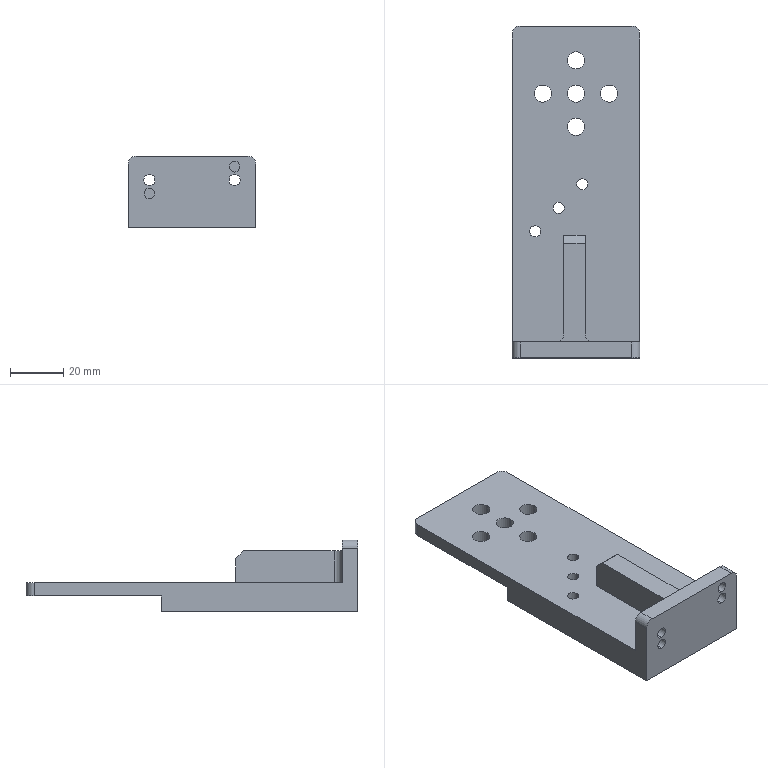Part | 1 solid | 47 faces | box 48 x 124.7 x 27 mm | volume 58099 mm3 | cylinder 30 | plane 17 | commonest cylinder face diameters 4.2 x10 6.5 x10 6 x6 4 x4
STEP:
#1=CARTESIAN_POINT('',(-17.439,-14.789,-27.));
#2=VERTEX_POINT('',#1);
#3=CARTESIAN_POINT('',(-13.239,-14.789,-27.));
#4=VERTEX_POINT('',#3);
#5=CARTESIAN_POINT('',(-15.339,-14.789,-27.));
#6=DIRECTION('',(0.,0.,1.));
#7=DIRECTION('',(1.,0.,0.));
#8=AXIS2_PLACEMENT_3D('',#5,#6,#7);
#9=CIRCLE('',#8,2.1);
#10=EDGE_CURVE('',#2,#4,#9,.T.);
#11=ORIENTED_EDGE('',*,*,#10,.F.);
#12=CARTESIAN_POINT('',(-17.439,-14.789,-16.));
#13=VERTEX_POINT('',#12);
#14=CARTESIAN_POINT('',(-17.439,-14.789,-27.));
#15=DIRECTION('',(0.,0.,1.));
#16=VECTOR('',#15,1000.);
#17=LINE('',#14,#16);
#18=EDGE_CURVE('',#13,#2,#17,.F.);
#19=ORIENTED_EDGE('',*,*,#18,.F.);
#20=CARTESIAN_POINT('',(-13.239,-14.789,-16.));
#21=VERTEX_POINT('',#20);
#22=CARTESIAN_POINT('',(-15.339,-14.789,-16.));
#23=DIRECTION('',(0.,0.,1.));
#24=DIRECTION('',(1.,0.,0.));
#25=AXIS2_PLACEMENT_3D('',#22,#23,#24);
#26=CIRCLE('',#25,2.1);
#27=EDGE_CURVE('',#13,#21,#26,.T.);
#28=ORIENTED_EDGE('',*,*,#27,.T.);
#29=CARTESIAN_POINT('',(-13.239,-14.789,-27.));
#30=DIRECTION('',(0.,0.,1.));
#31=VECTOR('',#30,1000.);
#32=LINE('',#29,#31);
#33=EDGE_CURVE('',#21,#4,#32,.F.);
#34=ORIENTED_EDGE('',*,*,#33,.T.);
#35=EDGE_LOOP('',(#11,#19,#28,#34));
#36=FACE_BOUND('',#35,.T.);
#37=CARTESIAN_POINT('',(-15.339,-14.789,-27.));
#38=DIRECTION('',(0.,0.,1.));
#39=DIRECTION('',(-1.,0.,0.));
#40=AXIS2_PLACEMENT_3D('',#37,#38,#39);
#41=CYLINDRICAL_SURFACE('',#40,2.1);
#42=ADVANCED_FACE('',(#36),#41,.F.);
#43=CARTESIAN_POINT('',(0.2388,2.889,-27.));
#44=VERTEX_POINT('',#43);
#45=CARTESIAN_POINT('',(4.439,2.889,-27.));
#46=VERTEX_POINT('',#45);
#47=CARTESIAN_POINT('',(2.339,2.889,-27.));
#48=DIRECTION('',(0.,0.,1.));
#49=DIRECTION('',(1.,0.,0.));
#50=AXIS2_PLACEMENT_3D('',#47,#48,#49);
#51=CIRCLE('',#50,2.1);
#52=EDGE_CURVE('',#44,#46,#51,.T.);
#53=ORIENTED_EDGE('',*,*,#52,.F.);
#54=CARTESIAN_POINT('',(0.2388,2.889,-16.));
#55=VERTEX_POINT('',#54);
#56=CARTESIAN_POINT('',(0.2388,2.889,-27.));
#57=DIRECTION('',(0.,0.,1.));
#58=VECTOR('',#57,1000.);
#59=LINE('',#56,#58);
#60=EDGE_CURVE('',#55,#44,#59,.F.);
#61=ORIENTED_EDGE('',*,*,#60,.F.);
#62=CARTESIAN_POINT('',(4.439,2.889,-16.));
#63=VERTEX_POINT('',#62);
#64=CARTESIAN_POINT('',(2.339,2.889,-16.));
#65=DIRECTION('',(0.,0.,1.));
#66=DIRECTION('',(1.,0.,0.));
#67=AXIS2_PLACEMENT_3D('',#64,#65,#66);
#68=CIRCLE('',#67,2.1);
#69=EDGE_CURVE('',#55,#63,#68,.T.);
#70=ORIENTED_EDGE('',*,*,#69,.T.);
#71=CARTESIAN_POINT('',(4.439,2.889,-27.));
#72=DIRECTION('',(0.,0.,1.));
#73=VECTOR('',#72,1000.);
#74=LINE('',#71,#73);
#75=EDGE_CURVE('',#63,#46,#74,.F.);
#76=ORIENTED_EDGE('',*,*,#75,.T.);
#77=EDGE_LOOP('',(#53,#61,#70,#76));
#78=FACE_BOUND('',#77,.T.);
#79=CARTESIAN_POINT('',(2.339,2.889,-27.));
#80=DIRECTION('',(0.,0.,1.));
#81=DIRECTION('',(-1.,0.,0.));
#82=AXIS2_PLACEMENT_3D('',#79,#80,#81);
#83=CYLINDRICAL_SURFACE('',#82,2.1);
#84=ADVANCED_FACE('',(#78),#83,.F.);
#85=CARTESIAN_POINT('',(-8.6,-5.95,-27.));
#86=VERTEX_POINT('',#85);
#87=CARTESIAN_POINT('',(-4.4,-5.95,-27.));
#88=VERTEX_POINT('',#87);
#89=CARTESIAN_POINT('',(-6.5,-5.95,-27.));
#90=DIRECTION('',(0.,0.,1.));
#91=DIRECTION('',(1.,0.,0.));
#92=AXIS2_PLACEMENT_3D('',#89,#90,#91);
#93=CIRCLE('',#92,2.1);
#94=EDGE_CURVE('',#86,#88,#93,.T.);
#95=ORIENTED_EDGE('',*,*,#94,.F.);
#96=CARTESIAN_POINT('',(-8.6,-5.95,-16.));
#97=VERTEX_POINT('',#96);
#98=CARTESIAN_POINT('',(-8.6,-5.95,-27.));
#99=DIRECTION('',(0.,0.,1.));
#100=VECTOR('',#99,1000.);
#101=LINE('',#98,#100);
#102=EDGE_CURVE('',#97,#86,#101,.F.);
#103=ORIENTED_EDGE('',*,*,#102,.F.);
#104=CARTESIAN_POINT('',(-4.4,-5.95,-16.));
#105=VERTEX_POINT('',#104);
#106=CARTESIAN_POINT('',(-6.5,-5.95,-16.));
#107=DIRECTION('',(0.,0.,1.));
#108=DIRECTION('',(1.,0.,0.));
#109=AXIS2_PLACEMENT_3D('',#106,#107,#108);
#110=CIRCLE('',#109,2.1);
#111=EDGE_CURVE('',#97,#105,#110,.T.);
#112=ORIENTED_EDGE('',*,*,#111,.T.);
#113=CARTESIAN_POINT('',(-4.4,-5.95,-27.));
#114=DIRECTION('',(0.,0.,1.));
#115=VECTOR('',#114,1000.);
#116=LINE('',#113,#115);
#117=EDGE_CURVE('',#105,#88,#116,.F.);
#118=ORIENTED_EDGE('',*,*,#117,.T.);
#119=EDGE_LOOP('',(#95,#103,#112,#118));
#120=FACE_BOUND('',#119,.T.);
#121=CARTESIAN_POINT('',(-6.5,-5.95,-27.));
#122=DIRECTION('',(0.,0.,1.));
#123=DIRECTION('',(-1.,0.,0.));
#124=AXIS2_PLACEMENT_3D('',#121,#122,#123);
#125=CYLINDRICAL_SURFACE('',#124,2.1);
#126=ADVANCED_FACE('',(#120),#125,.F.);
#127=CARTESIAN_POINT('',(16.,-59.35,-6.));
#128=VERTEX_POINT('',#127);
#129=CARTESIAN_POINT('',(16.,-59.35,-2.));
#130=VERTEX_POINT('',#129);
#131=CARTESIAN_POINT('',(16.,-59.35,-4.));
#132=DIRECTION('',(0.,-1.,0.));
#133=DIRECTION('',(0.,0.,1.));
#134=AXIS2_PLACEMENT_3D('',#131,#132,#133);
#135=CIRCLE('',#134,2.);
#136=EDGE_CURVE('',#128,#130,#135,.T.);
#137=ORIENTED_EDGE('',*,*,#136,.F.);
#138=CARTESIAN_POINT('',(16.,-62.35,-6.));
#139=VERTEX_POINT('',#138);
#140=CARTESIAN_POINT('',(16.,-59.35,-6.));
#141=DIRECTION('',(0.,-1.,0.));
#142=VECTOR('',#141,1000.);
#143=LINE('',#140,#142);
#144=EDGE_CURVE('',#139,#128,#143,.F.);
#145=ORIENTED_EDGE('',*,*,#144,.F.);
#146=CARTESIAN_POINT('',(16.,-62.35,-2.));
#147=VERTEX_POINT('',#146);
#148=CARTESIAN_POINT('',(16.,-62.35,-4.));
#149=DIRECTION('',(0.,-1.,0.));
#150=DIRECTION('',(0.,0.,1.));
#151=AXIS2_PLACEMENT_3D('',#148,#149,#150);
#152=CIRCLE('',#151,2.);
#153=EDGE_CURVE('',#139,#147,#152,.T.);
#154=ORIENTED_EDGE('',*,*,#153,.T.);
#155=CARTESIAN_POINT('',(16.,-59.35,-2.));
#156=DIRECTION('',(0.,-1.,0.));
#157=VECTOR('',#156,1000.);
#158=LINE('',#155,#157);
#159=EDGE_CURVE('',#147,#130,#158,.F.);
#160=ORIENTED_EDGE('',*,*,#159,.T.);
#161=EDGE_LOOP('',(#137,#145,#154,#160));
#162=FACE_BOUND('',#161,.T.);
#163=CARTESIAN_POINT('',(16.,-59.35,-4.));
#164=DIRECTION('',(0.,-1.,0.));
#165=DIRECTION('',(0.,0.,-1.));
#166=AXIS2_PLACEMENT_3D('',#163,#164,#165);
#167=CYLINDRICAL_SURFACE('',#166,2.);
#168=ADVANCED_FACE('',(#162),#167,.F.);
#169=CARTESIAN_POINT('',(-16.,-59.35,-16.));
#170=VERTEX_POINT('',#169);
#171=CARTESIAN_POINT('',(-16.,-59.35,-12.));
#172=VERTEX_POINT('',#171);
#173=CARTESIAN_POINT('',(-16.,-59.35,-14.));
#174=DIRECTION('',(0.,-1.,0.));
#175=DIRECTION('',(0.,0.,1.));
#176=AXIS2_PLACEMENT_3D('',#173,#174,#175);
#177=CIRCLE('',#176,2.);
#178=EDGE_CURVE('',#170,#172,#177,.T.);
#179=ORIENTED_EDGE('',*,*,#178,.F.);
#180=CARTESIAN_POINT('',(-16.,-62.35,-16.));
#181=VERTEX_POINT('',#180);
#182=CARTESIAN_POINT('',(-16.,-59.35,-16.));
#183=DIRECTION('',(0.,-1.,0.));
#184=VECTOR('',#183,1000.);
#185=LINE('',#182,#184);
#186=EDGE_CURVE('',#181,#170,#185,.F.);
#187=ORIENTED_EDGE('',*,*,#186,.F.);
#188=CARTESIAN_POINT('',(-16.,-62.35,-12.));
#189=VERTEX_POINT('',#188);
#190=CARTESIAN_POINT('',(-16.,-62.35,-14.));
#191=DIRECTION('',(0.,-1.,0.));
#192=DIRECTION('',(0.,0.,1.));
#193=AXIS2_PLACEMENT_3D('',#190,#191,#192);
#194=CIRCLE('',#193,2.);
#195=EDGE_CURVE('',#181,#189,#194,.T.);
#196=ORIENTED_EDGE('',*,*,#195,.T.);
#197=CARTESIAN_POINT('',(-16.,-59.35,-12.));
#198=DIRECTION('',(0.,-1.,0.));
#199=VECTOR('',#198,1000.);
#200=LINE('',#197,#199);
#201=EDGE_CURVE('',#189,#172,#200,.F.);
#202=ORIENTED_EDGE('',*,*,#201,.T.);
#203=EDGE_LOOP('',(#179,#187,#196,#202));
#204=FACE_BOUND('',#203,.T.);
#205=CARTESIAN_POINT('',(-16.,-59.35,-14.));
#206=DIRECTION('',(0.,-1.,0.));
#207=DIRECTION('',(0.,0.,-1.));
#208=AXIS2_PLACEMENT_3D('',#205,#206,#207);
#209=CYLINDRICAL_SURFACE('',#208,2.);
#210=ADVANCED_FACE('',(#204),#209,.F.);
#211=CARTESIAN_POINT('',(-3.25,49.45,-21.));
#212=VERTEX_POINT('',#211);
#213=CARTESIAN_POINT('',(3.25,49.45,-21.));
#214=VERTEX_POINT('',#213);
#215=CARTESIAN_POINT('',(0.,49.45,-21.));
#216=DIRECTION('',(0.,0.,1.));
#217=DIRECTION('',(1.,0.,0.));
#218=AXIS2_PLACEMENT_3D('',#215,#216,#217);
#219=CIRCLE('',#218,3.25);
#220=EDGE_CURVE('',#212,#214,#219,.T.);
#221=ORIENTED_EDGE('',*,*,#220,.F.);
#222=CARTESIAN_POINT('',(-3.25,49.45,-16.));
#223=VERTEX_POINT('',#222);
#224=CARTESIAN_POINT('',(-3.25,49.45,-27.));
#225=DIRECTION('',(0.,0.,1.));
#226=VECTOR('',#225,1000.);
#227=LINE('',#224,#226);
#228=EDGE_CURVE('',#223,#212,#227,.F.);
#229=ORIENTED_EDGE('',*,*,#228,.F.);
#230=CARTESIAN_POINT('',(3.25,49.45,-16.));
#231=VERTEX_POINT('',#230);
#232=CARTESIAN_POINT('',(0.,49.45,-16.));
#233=DIRECTION('',(0.,0.,1.));
#234=DIRECTION('',(1.,0.,0.));
#235=AXIS2_PLACEMENT_3D('',#232,#233,#234);
#236=CIRCLE('',#235,3.25);
#237=EDGE_CURVE('',#223,#231,#236,.T.);
#238=ORIENTED_EDGE('',*,*,#237,.T.);
#239=CARTESIAN_POINT('',(3.25,49.45,-27.));
#240=DIRECTION('',(0.,0.,1.));
#241=VECTOR('',#240,1000.);
#242=LINE('',#239,#241);
#243=EDGE_CURVE('',#231,#214,#242,.F.);
#244=ORIENTED_EDGE('',*,*,#243,.T.);
#245=EDGE_LOOP('',(#221,#229,#238,#244));
#246=FACE_BOUND('',#245,.T.);
#247=CARTESIAN_POINT('',(0.,49.45,-27.));
#248=DIRECTION('',(0.,0.,1.));
#249=DIRECTION('',(-1.,0.,0.));
#250=AXIS2_PLACEMENT_3D('',#247,#248,#249);
#251=CYLINDRICAL_SURFACE('',#250,3.25);
#252=ADVANCED_FACE('',(#246),#251,.F.);
#253=CARTESIAN_POINT('',(-15.75,36.95,-21.));
#254=VERTEX_POINT('',#253);
#255=CARTESIAN_POINT('',(-9.25,36.95,-21.));
#256=VERTEX_POINT('',#255);
#257=CARTESIAN_POINT('',(-12.5,36.95,-21.));
#258=DIRECTION('',(0.,0.,1.));
#259=DIRECTION('',(1.,0.,0.));
#260=AXIS2_PLACEMENT_3D('',#257,#258,#259);
#261=CIRCLE('',#260,3.25);
#262=EDGE_CURVE('',#254,#256,#261,.T.);
#263=ORIENTED_EDGE('',*,*,#262,.F.);
#264=CARTESIAN_POINT('',(-15.75,36.95,-16.));
#265=VERTEX_POINT('',#264);
#266=CARTESIAN_POINT('',(-15.75,36.95,-27.));
#267=DIRECTION('',(0.,0.,1.));
#268=VECTOR('',#267,1000.);
#269=LINE('',#266,#268);
#270=EDGE_CURVE('',#265,#254,#269,.F.);
#271=ORIENTED_EDGE('',*,*,#270,.F.);
#272=CARTESIAN_POINT('',(-9.25,36.95,-16.));
#273=VERTEX_POINT('',#272);
#274=CARTESIAN_POINT('',(-12.5,36.95,-16.));
#275=DIRECTION('',(0.,0.,1.));
#276=DIRECTION('',(1.,0.,0.));
#277=AXIS2_PLACEMENT_3D('',#274,#275,#276);
#278=CIRCLE('',#277,3.25);
#279=EDGE_CURVE('',#265,#273,#278,.T.);
#280=ORIENTED_EDGE('',*,*,#279,.T.);
#281=CARTESIAN_POINT('',(-9.25,36.95,-27.));
#282=DIRECTION('',(0.,0.,1.));
#283=VECTOR('',#282,1000.);
#284=LINE('',#281,#283);
#285=EDGE_CURVE('',#273,#256,#284,.F.);
#286=ORIENTED_EDGE('',*,*,#285,.T.);
#287=EDGE_LOOP('',(#263,#271,#280,#286));
#288=FACE_BOUND('',#287,.T.);
#289=CARTESIAN_POINT('',(-12.5,36.95,-27.));
#290=DIRECTION('',(0.,0.,1.));
#291=DIRECTION('',(-1.,0.,0.));
#292=AXIS2_PLACEMENT_3D('',#289,#290,#291);
#293=CYLINDRICAL_SURFACE('',#292,3.25);
#294=ADVANCED_FACE('',(#288),#293,.F.);
#295=CARTESIAN_POINT('',(9.25,36.95,-21.));
#296=VERTEX_POINT('',#295);
#297=CARTESIAN_POINT('',(15.75,36.95,-21.));
#298=VERTEX_POINT('',#297);
#299=CARTESIAN_POINT('',(12.5,36.95,-21.));
#300=DIRECTION('',(0.,0.,1.));
#301=DIRECTION('',(1.,0.,0.));
#302=AXIS2_PLACEMENT_3D('',#299,#300,#301);
#303=CIRCLE('',#302,3.25);
#304=EDGE_CURVE('',#296,#298,#303,.T.);
#305=ORIENTED_EDGE('',*,*,#304,.F.);
#306=CARTESIAN_POINT('',(9.25,36.95,-16.));
#307=VERTEX_POINT('',#306);
#308=CARTESIAN_POINT('',(9.25,36.95,-27.));
#309=DIRECTION('',(0.,0.,1.));
#310=VECTOR('',#309,1000.);
#311=LINE('',#308,#310);
#312=EDGE_CURVE('',#307,#296,#311,.F.);
#313=ORIENTED_EDGE('',*,*,#312,.F.);
#314=CARTESIAN_POINT('',(15.75,36.95,-16.));
#315=VERTEX_POINT('',#314);
#316=CARTESIAN_POINT('',(12.5,36.95,-16.));
#317=DIRECTION('',(0.,0.,1.));
#318=DIRECTION('',(1.,0.,0.));
#319=AXIS2_PLACEMENT_3D('',#316,#317,#318);
#320=CIRCLE('',#319,3.25);
#321=EDGE_CURVE('',#307,#315,#320,.T.);
#322=ORIENTED_EDGE('',*,*,#321,.T.);
#323=CARTESIAN_POINT('',(15.75,36.95,-27.));
#324=DIRECTION('',(0.,0.,1.));
#325=VECTOR('',#324,1000.);
#326=LINE('',#323,#325);
#327=EDGE_CURVE('',#315,#298,#326,.F.);
#328=ORIENTED_EDGE('',*,*,#327,.T.);
#329=EDGE_LOOP('',(#305,#313,#322,#328));
#330=FACE_BOUND('',#329,.T.);
#331=CARTESIAN_POINT('',(12.5,36.95,-27.));
#332=DIRECTION('',(0.,0.,1.));
#333=DIRECTION('',(-1.,0.,0.));
#334=AXIS2_PLACEMENT_3D('',#331,#332,#333);
#335=CYLINDRICAL_SURFACE('',#334,3.25);
#336=ADVANCED_FACE('',(#330),#335,.F.);
#337=CARTESIAN_POINT('',(-3.25,24.45,-21.));
#338=VERTEX_POINT('',#337);
#339=CARTESIAN_POINT('',(3.25,24.45,-21.));
#340=VERTEX_POINT('',#339);
#341=CARTESIAN_POINT('',(0.,24.45,-21.));
#342=DIRECTION('',(0.,0.,1.));
#343=DIRECTION('',(1.,0.,0.));
#344=AXIS2_PLACEMENT_3D('',#341,#342,#343);
#345=CIRCLE('',#344,3.25);
#346=EDGE_CURVE('',#338,#340,#345,.T.);
#347=ORIENTED_EDGE('',*,*,#346,.F.);
#348=CARTESIAN_POINT('',(-3.25,24.45,-16.));
#349=VERTEX_POINT('',#348);
#350=CARTESIAN_POINT('',(-3.25,24.45,-27.));
#351=DIRECTION('',(0.,0.,1.));
#352=VECTOR('',#351,1000.);
#353=LINE('',#350,#352);
#354=EDGE_CURVE('',#349,#338,#353,.F.);
#355=ORIENTED_EDGE('',*,*,#354,.F.);
#356=CARTESIAN_POINT('',(3.25,24.45,-16.));
#357=VERTEX_POINT('',#356);
#358=CARTESIAN_POINT('',(0.,24.45,-16.));
#359=DIRECTION('',(0.,0.,1.));
#360=DIRECTION('',(1.,0.,0.));
#361=AXIS2_PLACEMENT_3D('',#358,#359,#360);
#362=CIRCLE('',#361,3.25);
#363=EDGE_CURVE('',#349,#357,#362,.T.);
#364=ORIENTED_EDGE('',*,*,#363,.T.);
#365=CARTESIAN_POINT('',(3.25,24.45,-27.));
#366=DIRECTION('',(0.,0.,1.));
#367=VECTOR('',#366,1000.);
#368=LINE('',#365,#367);
#369=EDGE_CURVE('',#357,#340,#368,.F.);
#370=ORIENTED_EDGE('',*,*,#369,.T.);
#371=EDGE_LOOP('',(#347,#355,#364,#370));
#372=FACE_BOUND('',#371,.T.);
#373=CARTESIAN_POINT('',(0.,24.45,-27.));
#374=DIRECTION('',(0.,0.,1.));
#375=DIRECTION('',(-1.,0.,0.));
#376=AXIS2_PLACEMENT_3D('',#373,#374,#375);
#377=CYLINDRICAL_SURFACE('',#376,3.25);
#378=ADVANCED_FACE('',(#372),#377,.F.);
#379=CARTESIAN_POINT('',(-3.25,36.95,-21.));
#380=VERTEX_POINT('',#379);
#381=CARTESIAN_POINT('',(3.25,36.95,-21.));
#382=VERTEX_POINT('',#381);
#383=CARTESIAN_POINT('',(0.,36.95,-21.));
#384=DIRECTION('',(0.,0.,1.));
#385=DIRECTION('',(1.,0.,0.));
#386=AXIS2_PLACEMENT_3D('',#383,#384,#385);
#387=CIRCLE('',#386,3.25);
#388=EDGE_CURVE('',#380,#382,#387,.T.);
#389=ORIENTED_EDGE('',*,*,#388,.F.);
#390=CARTESIAN_POINT('',(-3.25,36.95,-16.));
#391=VERTEX_POINT('',#390);
#392=CARTESIAN_POINT('',(-3.25,36.95,-27.));
#393=DIRECTION('',(0.,0.,1.));
#394=VECTOR('',#393,1000.);
#395=LINE('',#392,#394);
#396=EDGE_CURVE('',#391,#380,#395,.F.);
#397=ORIENTED_EDGE('',*,*,#396,.F.);
#398=CARTESIAN_POINT('',(3.25,36.95,-16.));
#399=VERTEX_POINT('',#398);
#400=CARTESIAN_POINT('',(0.,36.95,-16.));
#401=DIRECTION('',(0.,0.,1.));
#402=DIRECTION('',(1.,0.,0.));
#403=AXIS2_PLACEMENT_3D('',#400,#401,#402);
#404=CIRCLE('',#403,3.25);
#405=EDGE_CURVE('',#391,#399,#404,.T.);
#406=ORIENTED_EDGE('',*,*,#405,.T.);
#407=CARTESIAN_POINT('',(3.25,36.95,-27.));
#408=DIRECTION('',(0.,0.,1.));
#409=VECTOR('',#408,1000.);
#410=LINE('',#407,#409);
#411=EDGE_CURVE('',#399,#382,#410,.F.);
#412=ORIENTED_EDGE('',*,*,#411,.T.);
#413=EDGE_LOOP('',(#389,#397,#406,#412));
#414=FACE_BOUND('',#413,.T.);
#415=CARTESIAN_POINT('',(0.,36.95,-27.));
#416=DIRECTION('',(0.,0.,1.));
#417=DIRECTION('',(-1.,0.,0.));
#418=AXIS2_PLACEMENT_3D('',#415,#416,#417);
#419=CYLINDRICAL_SURFACE('',#418,3.25);
#420=ADVANCED_FACE('',(#414),#419,.F.);
#421=CARTESIAN_POINT('',(16.,-62.35,-6.9));
#422=VERTEX_POINT('',#421);
#423=CARTESIAN_POINT('',(16.,-62.35,-11.1));
#424=VERTEX_POINT('',#423);
#425=CARTESIAN_POINT('',(16.,-62.35,-9.));
#426=DIRECTION('',(0.,1.,0.));
#427=DIRECTION('',(0.,0.,-1.));
#428=AXIS2_PLACEMENT_3D('',#425,#426,#427);
#429=CIRCLE('',#428,2.1);
#430=EDGE_CURVE('',#422,#424,#429,.T.);
#431=ORIENTED_EDGE('',*,*,#430,.F.);
#432=CARTESIAN_POINT('',(16.,-56.35,-6.9));
#433=VERTEX_POINT('',#432);
#434=CARTESIAN_POINT('',(16.,-62.35,-6.9));
#435=DIRECTION('',(0.,1.,0.));
#436=VECTOR('',#435,1000.);
#437=LINE('',#434,#436);
#438=EDGE_CURVE('',#433,#422,#437,.F.);
#439=ORIENTED_EDGE('',*,*,#438,.F.);
#440=CARTESIAN_POINT('',(16.,-56.35,-11.1));
#441=VERTEX_POINT('',#440);
#442=CARTESIAN_POINT('',(16.,-56.35,-9.));
#443=DIRECTION('',(0.,1.,0.));
#444=DIRECTION('',(0.,0.,-1.));
#445=AXIS2_PLACEMENT_3D('',#442,#443,#444);
#446=CIRCLE('',#445,2.1);
#447=EDGE_CURVE('',#433,#441,#446,.T.);
#448=ORIENTED_EDGE('',*,*,#447,.T.);
#449=CARTESIAN_POINT('',(16.,-62.35,-11.1));
#450=DIRECTION('',(0.,1.,0.));
#451=VECTOR('',#450,1000.);
#452=LINE('',#449,#451);
#453=EDGE_CURVE('',#441,#424,#452,.F.);
#454=ORIENTED_EDGE('',*,*,#453,.T.);
#455=EDGE_LOOP('',(#431,#439,#448,#454));
#456=FACE_BOUND('',#455,.T.);
#457=CARTESIAN_POINT('',(16.,-62.35,-9.));
#458=DIRECTION('',(0.,1.,0.));
#459=DIRECTION('',(0.,0.,1.));
#460=AXIS2_PLACEMENT_3D('',#457,#458,#459);
#461=CYLINDRICAL_SURFACE('',#460,2.1);
#462=ADVANCED_FACE('',(#456),#461,.F.);
#463=CARTESIAN_POINT('',(-16.,-62.35,-6.9));
#464=VERTEX_POINT('',#463);
#465=CARTESIAN_POINT('',(-16.,-62.35,-11.1));
#466=VERTEX_POINT('',#465);
#467=CARTESIAN_POINT('',(-16.,-62.35,-9.));
#468=DIRECTION('',(0.,1.,0.));
#469=DIRECTION('',(0.,0.,-1.));
#470=AXIS2_PLACEMENT_3D('',#467,#468,#469);
#471=CIRCLE('',#470,2.1);
#472=EDGE_CURVE('',#464,#466,#471,.T.);
#473=ORIENTED_EDGE('',*,*,#472,.F.);
#474=CARTESIAN_POINT('',(-16.,-56.35,-6.9));
#475=VERTEX_POINT('',#474);
#476=CARTESIAN_POINT('',(-16.,-62.35,-6.9));
#477=DIRECTION('',(0.,1.,0.));
#478=VECTOR('',#477,1000.);
#479=LINE('',#476,#478);
#480=EDGE_CURVE('',#475,#464,#479,.F.);
#481=ORIENTED_EDGE('',*,*,#480,.F.);
#482=CARTESIAN_POINT('',(-16.,-56.35,-11.1));
#483=VERTEX_POINT('',#482);
#484=CARTESIAN_POINT('',(-16.,-56.35,-9.));
#485=DIRECTION('',(0.,1.,0.));
#486=DIRECTION('',(0.,0.,-1.));
#487=AXIS2_PLACEMENT_3D('',#484,#485,#486);
#488=CIRCLE('',#487,2.1);
#489=EDGE_CURVE('',#475,#483,#488,.T.);
#490=ORIENTED_EDGE('',*,*,#489,.T.);
#491=CARTESIAN_POINT('',(-16.,-62.35,-11.1));
#492=DIRECTION('',(0.,1.,0.));
#493=VECTOR('',#492,1000.);
#494=LINE('',#491,#493);
#495=EDGE_CURVE('',#483,#466,#494,.F.);
#496=ORIENTED_EDGE('',*,*,#495,.T.);
#497=EDGE_LOOP('',(#473,#481,#490,#496));
#498=FACE_BOUND('',#497,.T.);
#499=CARTESIAN_POINT('',(-16.,-62.35,-9.));
#500=DIRECTION('',(0.,1.,0.));
#501=DIRECTION('',(0.,0.,1.));
#502=AXIS2_PLACEMENT_3D('',#499,#500,#501);
#503=CYLINDRICAL_SURFACE('',#502,2.1);
#504=ADVANCED_FACE('',(#498),#503,.F.);
#505=CARTESIAN_POINT('',(-15.339,-14.789,-16.));
#506=DIRECTION('',(0.,0.,1.));
#507=DIRECTION('',(1.,0.,0.));
#508=AXIS2_PLACEMENT_3D('',#505,#506,#507);
#509=CIRCLE('',#508,2.1);
#510=EDGE_CURVE('',#21,#13,#509,.T.);
#511=ORIENTED_EDGE('',*,*,#510,.F.);
#512=ORIENTED_EDGE('',*,*,#27,.F.);
#513=EDGE_LOOP('',(#511,#512));
#514=FACE_BOUND('',#513,.T.);
#515=CARTESIAN_POINT('',(2.339,2.889,-16.));
#516=DIRECTION('',(0.,0.,1.));
#517=DIRECTION('',(1.,0.,0.));
#518=AXIS2_PLACEMENT_3D('',#515,#516,#517);
#519=CIRCLE('',#518,2.1);
#520=EDGE_CURVE('',#63,#55,#519,.T.);
#521=ORIENTED_EDGE('',*,*,#520,.F.);
#522=ORIENTED_EDGE('',*,*,#69,.F.);
#523=EDGE_LOOP('',(#521,#522));
#524=FACE_BOUND('',#523,.T.);
#525=CARTESIAN_POINT('',(-6.5,-5.95,-16.));
#526=DIRECTION('',(0.,0.,1.));
#527=DIRECTION('',(1.,0.,0.));
#528=AXIS2_PLACEMENT_3D('',#525,#526,#527);
#529=CIRCLE('',#528,2.1);
#530=EDGE_CURVE('',#105,#97,#529,.T.);
#531=ORIENTED_EDGE('',*,*,#530,.F.);
#532=ORIENTED_EDGE('',*,*,#111,.F.);
#533=EDGE_LOOP('',(#531,#532));
#534=FACE_BOUND('',#533,.T.);
#535=CARTESIAN_POINT('',(0.,49.45,-16.));
#536=DIRECTION('',(0.,0.,1.));
#537=DIRECTION('',(1.,0.,0.));
#538=AXIS2_PLACEMENT_3D('',#535,#536,#537);
#539=CIRCLE('',#538,3.25);
#540=EDGE_CURVE('',#231,#223,#539,.T.);
#541=ORIENTED_EDGE('',*,*,#540,.F.);
#542=ORIENTED_EDGE('',*,*,#237,.F.);
#543=EDGE_LOOP('',(#541,#542));
#544=FACE_BOUND('',#543,.T.);
#545=CARTESIAN_POINT('',(-12.5,36.95,-16.));
#546=DIRECTION('',(0.,0.,1.));
#547=DIRECTION('',(1.,0.,0.));
#548=AXIS2_PLACEMENT_3D('',#545,#546,#547);
#549=CIRCLE('',#548,3.25);
#550=EDGE_CURVE('',#273,#265,#549,.T.);
#551=ORIENTED_EDGE('',*,*,#550,.F.);
#552=ORIENTED_EDGE('',*,*,#279,.F.);
#553=EDGE_LOOP('',(#551,#552));
#554=FACE_BOUND('',#553,.T.);
#555=CARTESIAN_POINT('',(12.5,36.95,-16.));
#556=DIRECTION('',(0.,0.,1.));
#557=DIRECTION('',(1.,0.,0.));
#558=AXIS2_PLACEMENT_3D('',#555,#556,#557);
#559=CIRCLE('',#558,3.25);
#560=EDGE_CURVE('',#315,#307,#559,.T.);
#561=ORIENTED_EDGE('',*,*,#560,.F.);
#562=ORIENTED_EDGE('',*,*,#321,.F.);
#563=EDGE_LOOP('',(#561,#562));
#564=FACE_BOUND('',#563,.T.);
#565=CARTESIAN_POINT('',(0.,24.45,-16.));
#566=DIRECTION('',(0.,0.,1.));
#567=DIRECTION('',(1.,0.,0.));
#568=AXIS2_PLACEMENT_3D('',#565,#566,#567);
#569=CIRCLE('',#568,3.25);
#570=EDGE_CURVE('',#357,#349,#569,.T.);
#571=ORIENTED_EDGE('',*,*,#570,.F.);
#572=ORIENTED_EDGE('',*,*,#363,.F.);
#573=EDGE_LOOP('',(#571,#572));
#574=FACE_BOUND('',#573,.T.);
#575=CARTESIAN_POINT('',(0.,36.95,-16.));
#576=DIRECTION('',(0.,0.,1.));
#577=DIRECTION('',(1.,0.,0.));
#578=AXIS2_PLACEMENT_3D('',#575,#576,#577);
#579=CIRCLE('',#578,3.25);
#580=EDGE_CURVE('',#399,#391,#579,.T.);
#581=ORIENTED_EDGE('',*,*,#580,.F.);
#582=ORIENTED_EDGE('',*,*,#405,.F.);
#583=EDGE_LOOP('',(#581,#582));
#584=FACE_BOUND('',#583,.T.);
#585=CARTESIAN_POINT('',(-7.573,-56.35,-16.));
#586=VERTEX_POINT('',#585);
#587=CARTESIAN_POINT('',(-24.,-56.35,-16.));
#588=VERTEX_POINT('',#587);
#589=CARTESIAN_POINT('',(-24.,-56.35,-16.));
#590=DIRECTION('',(-1.,0.,0.));
#591=VECTOR('',#590,1000.);
#592=LINE('',#589,#591);
#593=EDGE_CURVE('',#586,#588,#592,.T.);
#594=ORIENTED_EDGE('',*,*,#593,.F.);
#595=CARTESIAN_POINT('',(-4.573,-53.35,-16.));
#596=VERTEX_POINT('',#595);
#597=CARTESIAN_POINT('',(-7.573,-53.35,-16.));
#598=DIRECTION('',(0.,0.,1.));
#599=DIRECTION('',(1.,0.,0.));
#600=AXIS2_PLACEMENT_3D('',#597,#598,#599);
#601=CIRCLE('',#600,3.);
#602=EDGE_CURVE('',#586,#596,#601,.T.);
#603=ORIENTED_EDGE('',*,*,#602,.T.);
#604=CARTESIAN_POINT('',(-4.573,-16.35,-16.));
#605=VERTEX_POINT('',#604);
#606=CARTESIAN_POINT('',(-4.573,-56.35,-16.));
#607=DIRECTION('',(0.,-1.,0.));
#608=VECTOR('',#607,1000.);
#609=LINE('',#606,#608);
#610=EDGE_CURVE('',#605,#596,#609,.T.);
#611=ORIENTED_EDGE('',*,*,#610,.F.);
#612=CARTESIAN_POINT('',(3.427,-16.35,-16.));
#613=VERTEX_POINT('',#612);
#614=CARTESIAN_POINT('',(-4.573,-16.35,-16.));
#615=DIRECTION('',(-1.,0.,0.));
#616=VECTOR('',#615,1000.);
#617=LINE('',#614,#616);
#618=EDGE_CURVE('',#613,#605,#617,.T.);
#619=ORIENTED_EDGE('',*,*,#618,.F.);
#620=CARTESIAN_POINT('',(3.427,-53.35,-16.));
#621=VERTEX_POINT('',#620);
#622=CARTESIAN_POINT('',(3.427,-56.35,-16.));
#623=DIRECTION('',(0.,1.,0.));
#624=VECTOR('',#623,1000.);
#625=LINE('',#622,#624);
#626=EDGE_CURVE('',#621,#613,#625,.T.);
#627=ORIENTED_EDGE('',*,*,#626,.F.);
#628=CARTESIAN_POINT('',(6.427,-56.35,-16.));
#629=VERTEX_POINT('',#628);
#630=CARTESIAN_POINT('',(6.427,-53.35,-16.));
#631=DIRECTION('',(0.,0.,1.));
#632=DIRECTION('',(1.,0.,0.));
#633=AXIS2_PLACEMENT_3D('',#630,#631,#632);
#634=CIRCLE('',#633,3.);
#635=EDGE_CURVE('',#621,#629,#634,.T.);
#636=ORIENTED_EDGE('',*,*,#635,.T.);
#637=CARTESIAN_POINT('',(24.,-56.35,-16.));
#638=VERTEX_POINT('',#637);
#639=CARTESIAN_POINT('',(-24.,-56.35,-16.));
#640=DIRECTION('',(-1.,0.,0.));
#641=VECTOR('',#640,1000.);
#642=LINE('',#639,#641);
#643=EDGE_CURVE('',#638,#629,#642,.T.);
#644=ORIENTED_EDGE('',*,*,#643,.F.);
#645=CARTESIAN_POINT('',(24.,59.35,-16.));
#646=VERTEX_POINT('',#645);
#647=CARTESIAN_POINT('',(24.,-62.35,-16.));
#648=DIRECTION('',(0.,-1.,0.));
#649=VECTOR('',#648,1000.);
#650=LINE('',#647,#649);
#651=EDGE_CURVE('',#646,#638,#650,.T.);
#652=ORIENTED_EDGE('',*,*,#651,.F.);
#653=CARTESIAN_POINT('',(21.,62.35,-16.));
#654=VERTEX_POINT('',#653);
#655=CARTESIAN_POINT('',(21.,59.35,-16.));
#656=DIRECTION('',(0.,0.,1.));
#657=DIRECTION('',(1.,0.,0.));
#658=AXIS2_PLACEMENT_3D('',#655,#656,#657);
#659=CIRCLE('',#658,3.);
#660=EDGE_CURVE('',#646,#654,#659,.T.);
#661=ORIENTED_EDGE('',*,*,#660,.T.);
#662=CARTESIAN_POINT('',(-21.,62.35,-16.));
#663=VERTEX_POINT('',#662);
#664=CARTESIAN_POINT('',(24.,62.35,-16.));
#665=DIRECTION('',(1.,0.,0.));
#666=VECTOR('',#665,1000.);
#667=LINE('',#664,#666);
#668=EDGE_CURVE('',#663,#654,#667,.T.);
#669=ORIENTED_EDGE('',*,*,#668,.F.);
#670=CARTESIAN_POINT('',(-24.,59.35,-16.));
#671=VERTEX_POINT('',#670);
#672=CARTESIAN_POINT('',(-21.,59.35,-16.));
#673=DIRECTION('',(0.,0.,1.));
#674=DIRECTION('',(1.,0.,0.));
#675=AXIS2_PLACEMENT_3D('',#672,#673,#674);
#676=CIRCLE('',#675,3.);
#677=EDGE_CURVE('',#663,#671,#676,.T.);
#678=ORIENTED_EDGE('',*,*,#677,.T.);
#679=CARTESIAN_POINT('',(-24.,-62.35,-16.));
#680=DIRECTION('',(0.,1.,0.));
#681=VECTOR('',#680,1000.);
#682=LINE('',#679,#681);
#683=EDGE_CURVE('',#588,#671,#682,.T.);
#684=ORIENTED_EDGE('',*,*,#683,.F.);
#685=EDGE_LOOP('',(#594,#603,#611,#619,#627,#636,#644,#652,#661,#669,#678,#684));
#686=FACE_BOUND('',#685,.T.);
#687=CARTESIAN_POINT('',(24.,-62.35,-16.));
#688=DIRECTION('',(0.,0.,1.));
#689=DIRECTION('',(-1.,0.,0.));
#690=AXIS2_PLACEMENT_3D('',#687,#688,#689);
#691=PLANE('',#690);
#692=ADVANCED_FACE('',(#514,#524,#534,#544,#554,#564,#574,#584,#686),#691,.T.);
#693=CARTESIAN_POINT('',(16.,-56.35,-9.));
#694=DIRECTION('',(0.,1.,0.));
#695=DIRECTION('',(0.,0.,-1.));
#696=AXIS2_PLACEMENT_3D('',#693,#694,#695);
#697=CIRCLE('',#696,2.1);
#698=EDGE_CURVE('',#441,#433,#697,.T.);
#699=ORIENTED_EDGE('',*,*,#698,.F.);
#700=ORIENTED_EDGE('',*,*,#447,.F.);
#701=EDGE_LOOP('',(#699,#700));
#702=FACE_BOUND('',#701,.T.);
#703=CARTESIAN_POINT('',(-16.,-56.35,-9.));
#704=DIRECTION('',(0.,1.,0.));
#705=DIRECTION('',(0.,0.,-1.));
#706=AXIS2_PLACEMENT_3D('',#703,#704,#705);
#707=CIRCLE('',#706,2.1);
#708=EDGE_CURVE('',#483,#475,#707,.T.);
#709=ORIENTED_EDGE('',*,*,#708,.F.);
#710=ORIENTED_EDGE('',*,*,#489,.F.);
#711=EDGE_LOOP('',(#709,#710));
#712=FACE_BOUND('',#711,.T.);
#713=CARTESIAN_POINT('',(-7.573,-56.35,-4.));
#714=VERTEX_POINT('',#713);
#715=CARTESIAN_POINT('',(6.427,-56.35,-4.));
#716=VERTEX_POINT('',#715);
#717=CARTESIAN_POINT('',(-4.573,-56.35,-4.));
#718=DIRECTION('',(1.,0.,0.));
#719=VECTOR('',#718,1000.);
#720=LINE('',#717,#719);
#721=EDGE_CURVE('',#714,#716,#720,.T.);
#722=ORIENTED_EDGE('',*,*,#721,.F.);
#723=CARTESIAN_POINT('',(-7.573,-56.35,-16.));
#724=DIRECTION('',(0.,0.,-1.));
#725=VECTOR('',#724,1000.);
#726=LINE('',#723,#725);
#727=EDGE_CURVE('',#714,#586,#726,.T.);
#728=ORIENTED_EDGE('',*,*,#727,.T.);
#729=ORIENTED_EDGE('',*,*,#593,.T.);
#730=CARTESIAN_POINT('',(-24.,-56.35,-3.));
#731=VERTEX_POINT('',#730);
#732=CARTESIAN_POINT('',(-24.,-56.35,0.));
#733=DIRECTION('',(0.,0.,-1.));
#734=VECTOR('',#733,1000.);
#735=LINE('',#732,#734);
#736=EDGE_CURVE('',#731,#588,#735,.T.);
#737=ORIENTED_EDGE('',*,*,#736,.F.);
#738=CARTESIAN_POINT('',(-21.,-56.35,0.));
#739=VERTEX_POINT('',#738);
#740=CARTESIAN_POINT('',(-21.,-56.35,-3.));
#741=DIRECTION('',(0.,1.,0.));
#742=DIRECTION('',(0.,0.,1.));
#743=AXIS2_PLACEMENT_3D('',#740,#741,#742);
#744=CIRCLE('',#743,3.);
#745=EDGE_CURVE('',#731,#739,#744,.T.);
#746=ORIENTED_EDGE('',*,*,#745,.T.);
#747=CARTESIAN_POINT('',(21.,-56.35,0.));
#748=VERTEX_POINT('',#747);
#749=CARTESIAN_POINT('',(-24.,-56.35,0.));
#750=DIRECTION('',(-1.,0.,0.));
#751=VECTOR('',#750,1000.);
#752=LINE('',#749,#751);
#753=EDGE_CURVE('',#748,#739,#752,.T.);
#754=ORIENTED_EDGE('',*,*,#753,.F.);
#755=CARTESIAN_POINT('',(24.,-56.35,-3.));
#756=VERTEX_POINT('',#755);
#757=CARTESIAN_POINT('',(21.,-56.35,-3.));
#758=DIRECTION('',(0.,1.,0.));
#759=DIRECTION('',(0.,0.,1.));
#760=AXIS2_PLACEMENT_3D('',#757,#758,#759);
#761=CIRCLE('',#760,3.);
#762=EDGE_CURVE('',#748,#756,#761,.T.);
#763=ORIENTED_EDGE('',*,*,#762,.T.);
#764=CARTESIAN_POINT('',(24.,-56.35,0.));
#765=DIRECTION('',(0.,0.,-1.));
#766=VECTOR('',#765,1000.);
#767=LINE('',#764,#766);
#768=EDGE_CURVE('',#756,#638,#767,.T.);
#769=ORIENTED_EDGE('',*,*,#768,.T.);
#770=ORIENTED_EDGE('',*,*,#643,.T.);
#771=CARTESIAN_POINT('',(6.427,-56.35,-4.));
#772=DIRECTION('',(0.,0.,1.));
#773=VECTOR('',#772,1000.);
#774=LINE('',#771,#773);
#775=EDGE_CURVE('',#629,#716,#774,.T.);
#776=ORIENTED_EDGE('',*,*,#775,.T.);
#777=EDGE_LOOP('',(#722,#728,#729,#737,#746,#754,#763,#769,#770,#776));
#778=FACE_BOUND('',#777,.T.);
#779=CARTESIAN_POINT('',(-24.,-56.35,0.));
#780=DIRECTION('',(0.,-1.,0.));
#781=DIRECTION('',(0.,0.,-1.));
#782=AXIS2_PLACEMENT_3D('',#779,#780,#781);
#783=PLANE('',#782);
#784=ADVANCED_FACE('',(#702,#712,#778),#783,.F.);
#785=CARTESIAN_POINT('',(0.,49.45,-21.));
#786=DIRECTION('',(0.,0.,1.));
#787=DIRECTION('',(1.,0.,0.));
#788=AXIS2_PLACEMENT_3D('',#785,#786,#787);
#789=CIRCLE('',#788,3.25);
#790=EDGE_CURVE('',#214,#212,#789,.T.);
#791=ORIENTED_EDGE('',*,*,#790,.T.);
#792=ORIENTED_EDGE('',*,*,#220,.T.);
#793=EDGE_LOOP('',(#791,#792));
#794=FACE_BOUND('',#793,.T.);
#795=CARTESIAN_POINT('',(-12.5,36.95,-21.));
#796=DIRECTION('',(0.,0.,1.));
#797=DIRECTION('',(1.,0.,0.));
#798=AXIS2_PLACEMENT_3D('',#795,#796,#797);
#799=CIRCLE('',#798,3.25);
#800=EDGE_CURVE('',#256,#254,#799,.T.);
#801=ORIENTED_EDGE('',*,*,#800,.T.);
#802=ORIENTED_EDGE('',*,*,#262,.T.);
#803=EDGE_LOOP('',(#801,#802));
#804=FACE_BOUND('',#803,.T.);
#805=CARTESIAN_POINT('',(12.5,36.95,-21.));
#806=DIRECTION('',(0.,0.,1.));
#807=DIRECTION('',(1.,0.,0.));
#808=AXIS2_PLACEMENT_3D('',#805,#806,#807);
#809=CIRCLE('',#808,3.25);
#810=EDGE_CURVE('',#298,#296,#809,.T.);
#811=ORIENTED_EDGE('',*,*,#810,.T.);
#812=ORIENTED_EDGE('',*,*,#304,.T.);
#813=EDGE_LOOP('',(#811,#812));
#814=FACE_BOUND('',#813,.T.);
#815=CARTESIAN_POINT('',(0.,24.45,-21.));
#816=DIRECTION('',(0.,0.,1.));
#817=DIRECTION('',(1.,0.,0.));
#818=AXIS2_PLACEMENT_3D('',#815,#816,#817);
#819=CIRCLE('',#818,3.25);
#820=EDGE_CURVE('',#340,#338,#819,.T.);
#821=ORIENTED_EDGE('',*,*,#820,.T.);
#822=ORIENTED_EDGE('',*,*,#346,.T.);
#823=EDGE_LOOP('',(#821,#822));
#824=FACE_BOUND('',#823,.T.);
#825=CARTESIAN_POINT('',(0.,36.95,-21.));
#826=DIRECTION('',(0.,0.,1.));
#827=DIRECTION('',(1.,0.,0.));
#828=AXIS2_PLACEMENT_3D('',#825,#826,#827);
#829=CIRCLE('',#828,3.25);
#830=EDGE_CURVE('',#382,#380,#829,.T.);
#831=ORIENTED_EDGE('',*,*,#830,.T.);
#832=ORIENTED_EDGE('',*,*,#388,.T.);
#833=EDGE_LOOP('',(#831,#832));
#834=FACE_BOUND('',#833,.T.);
#835=CARTESIAN_POINT('',(-21.,62.35,-21.));
#836=VERTEX_POINT('',#835);
#837=CARTESIAN_POINT('',(21.,62.35,-21.));
#838=VERTEX_POINT('',#837);
#839=CARTESIAN_POINT('',(24.,62.35,-21.));
#840=DIRECTION('',(1.,0.,0.));
#841=VECTOR('',#840,1000.);
#842=LINE('',#839,#841);
#843=EDGE_CURVE('',#836,#838,#842,.T.);
#844=ORIENTED_EDGE('',*,*,#843,.T.);
#845=CARTESIAN_POINT('',(24.,59.35,-21.));
#846=VERTEX_POINT('',#845);
#847=CARTESIAN_POINT('',(21.,59.35,-21.));
#848=DIRECTION('',(0.,0.,-1.));
#849=DIRECTION('',(1.,0.,0.));
#850=AXIS2_PLACEMENT_3D('',#847,#848,#849);
#851=CIRCLE('',#850,3.);
#852=EDGE_CURVE('',#838,#846,#851,.T.);
#853=ORIENTED_EDGE('',*,*,#852,.T.);
#854=CARTESIAN_POINT('',(24.,11.55,-21.));
#855=VERTEX_POINT('',#854);
#856=CARTESIAN_POINT('',(24.,-62.35,-21.));
#857=DIRECTION('',(0.,-1.,0.));
#858=VECTOR('',#857,1000.);
#859=LINE('',#856,#858);
#860=EDGE_CURVE('',#846,#855,#859,.T.);
#861=ORIENTED_EDGE('',*,*,#860,.T.);
#862=CARTESIAN_POINT('',(-24.,11.55,-21.));
#863=VERTEX_POINT('',#862);
#864=CARTESIAN_POINT('',(24.,11.55,-21.));
#865=DIRECTION('',(1.,0.,0.));
#866=VECTOR('',#865,1000.);
#867=LINE('',#864,#866);
#868=EDGE_CURVE('',#863,#855,#867,.T.);
#869=ORIENTED_EDGE('',*,*,#868,.F.);
#870=CARTESIAN_POINT('',(-24.,59.35,-21.));
#871=VERTEX_POINT('',#870);
#872=CARTESIAN_POINT('',(-24.,-62.35,-21.));
#873=DIRECTION('',(0.,1.,0.));
#874=VECTOR('',#873,1000.);
#875=LINE('',#872,#874);
#876=EDGE_CURVE('',#863,#871,#875,.T.);
#877=ORIENTED_EDGE('',*,*,#876,.T.);
#878=CARTESIAN_POINT('',(-21.,59.35,-21.));
#879=DIRECTION('',(0.,0.,-1.));
#880=DIRECTION('',(1.,0.,0.));
#881=AXIS2_PLACEMENT_3D('',#878,#879,#880);
#882=CIRCLE('',#881,3.);
#883=EDGE_CURVE('',#871,#836,#882,.T.);
#884=ORIENTED_EDGE('',*,*,#883,.T.);
#885=EDGE_LOOP('',(#844,#853,#861,#869,#877,#884));
#886=FACE_BOUND('',#885,.T.);
#887=CARTESIAN_POINT('',(24.,-62.35,-21.));
#888=DIRECTION('',(0.,0.,1.));
#889=DIRECTION('',(-1.,0.,0.));
#890=AXIS2_PLACEMENT_3D('',#887,#888,#889);
#891=PLANE('',#890);
#892=ADVANCED_FACE('',(#794,#804,#814,#824,#834,#886),#891,.F.);
#893=ORIENTED_EDGE('',*,*,#768,.F.);
#894=CARTESIAN_POINT('',(24.,-62.35,-3.));
#895=VERTEX_POINT('',#894);
#896=CARTESIAN_POINT('',(24.,-62.35,-3.));
#897=DIRECTION('',(0.,-1.,0.));
#898=VECTOR('',#897,1000.);
#899=LINE('',#896,#898);
#900=EDGE_CURVE('',#756,#895,#899,.T.);
#901=ORIENTED_EDGE('',*,*,#900,.T.);
#902=CARTESIAN_POINT('',(24.,-62.35,-27.));
#903=VERTEX_POINT('',#902);
#904=CARTESIAN_POINT('',(24.,-62.35,-21.));
#905=DIRECTION('',(0.,0.,1.));
#906=VECTOR('',#905,1000.);
#907=LINE('',#904,#906);
#908=EDGE_CURVE('',#903,#895,#907,.T.);
#909=ORIENTED_EDGE('',*,*,#908,.F.);
#910=CARTESIAN_POINT('',(24.,11.55,-27.));
#911=VERTEX_POINT('',#910);
#912=CARTESIAN_POINT('',(24.,-62.35,-27.));
#913=DIRECTION('',(0.,-1.,0.));
#914=VECTOR('',#913,1000.);
#915=LINE('',#912,#914);
#916=EDGE_CURVE('',#911,#903,#915,.T.);
#917=ORIENTED_EDGE('',*,*,#916,.F.);
#918=CARTESIAN_POINT('',(24.,11.55,-27.));
#919=DIRECTION('',(0.,0.,1.));
#920=VECTOR('',#919,1000.);
#921=LINE('',#918,#920);
#922=EDGE_CURVE('',#911,#855,#921,.T.);
#923=ORIENTED_EDGE('',*,*,#922,.T.);
#924=ORIENTED_EDGE('',*,*,#860,.F.);
#925=CARTESIAN_POINT('',(24.,59.35,-21.));
#926=DIRECTION('',(0.,0.,1.));
#927=VECTOR('',#926,1000.);
#928=LINE('',#925,#927);
#929=EDGE_CURVE('',#846,#646,#928,.T.);
#930=ORIENTED_EDGE('',*,*,#929,.T.);
#931=ORIENTED_EDGE('',*,*,#651,.T.);
#932=EDGE_LOOP('',(#893,#901,#909,#917,#923,#924,#930,#931));
#933=FACE_BOUND('',#932,.T.);
#934=CARTESIAN_POINT('',(24.,-62.35,-21.));
#935=DIRECTION('',(-1.,0.,0.));
#936=DIRECTION('',(0.,-1.,0.));
#937=AXIS2_PLACEMENT_3D('',#934,#935,#936);
#938=PLANE('',#937);
#939=ADVANCED_FACE('',(#933),#938,.F.);
#940=CARTESIAN_POINT('',(16.,-62.35,-4.));
#941=DIRECTION('',(0.,-1.,0.));
#942=DIRECTION('',(0.,0.,1.));
#943=AXIS2_PLACEMENT_3D('',#940,#941,#942);
#944=CIRCLE('',#943,2.);
#945=EDGE_CURVE('',#147,#139,#944,.T.);
#946=ORIENTED_EDGE('',*,*,#945,.F.);
#947=ORIENTED_EDGE('',*,*,#153,.F.);
#948=EDGE_LOOP('',(#946,#947));
#949=FACE_BOUND('',#948,.T.);
#950=CARTESIAN_POINT('',(-16.,-62.35,-14.));
#951=DIRECTION('',(0.,-1.,0.));
#952=DIRECTION('',(0.,0.,1.));
#953=AXIS2_PLACEMENT_3D('',#950,#951,#952);
#954=CIRCLE('',#953,2.);
#955=EDGE_CURVE('',#189,#181,#954,.T.);
#956=ORIENTED_EDGE('',*,*,#955,.F.);
#957=ORIENTED_EDGE('',*,*,#195,.F.);
#958=EDGE_LOOP('',(#956,#957));
#959=FACE_BOUND('',#958,.T.);
#960=CARTESIAN_POINT('',(16.,-62.35,-9.));
#961=DIRECTION('',(0.,1.,0.));
#962=DIRECTION('',(0.,0.,-1.));
#963=AXIS2_PLACEMENT_3D('',#960,#961,#962);
#964=CIRCLE('',#963,2.1);
#965=EDGE_CURVE('',#424,#422,#964,.T.);
#966=ORIENTED_EDGE('',*,*,#965,.T.);
#967=ORIENTED_EDGE('',*,*,#430,.T.);
#968=EDGE_LOOP('',(#966,#967));
#969=FACE_BOUND('',#968,.T.);
#970=CARTESIAN_POINT('',(-16.,-62.35,-9.));
#971=DIRECTION('',(0.,1.,0.));
#972=DIRECTION('',(0.,0.,-1.));
#973=AXIS2_PLACEMENT_3D('',#970,#971,#972);
#974=CIRCLE('',#973,2.1);
#975=EDGE_CURVE('',#466,#464,#974,.T.);
#976=ORIENTED_EDGE('',*,*,#975,.T.);
#977=ORIENTED_EDGE('',*,*,#472,.T.);
#978=EDGE_LOOP('',(#976,#977));
#979=FACE_BOUND('',#978,.T.);
#980=CARTESIAN_POINT('',(-21.,-62.35,0.));
#981=VERTEX_POINT('',#980);
#982=CARTESIAN_POINT('',(21.,-62.35,0.));
#983=VERTEX_POINT('',#982);
#984=CARTESIAN_POINT('',(-24.,-62.35,0.));
#985=DIRECTION('',(1.,0.,0.));
#986=VECTOR('',#985,1000.);
#987=LINE('',#984,#986);
#988=EDGE_CURVE('',#981,#983,#987,.T.);
#989=ORIENTED_EDGE('',*,*,#988,.F.);
#990=CARTESIAN_POINT('',(-24.,-62.35,-3.));
#991=VERTEX_POINT('',#990);
#992=CARTESIAN_POINT('',(-21.,-62.35,-3.));
#993=DIRECTION('',(0.,-1.,0.));
#994=DIRECTION('',(0.,0.,-1.));
#995=AXIS2_PLACEMENT_3D('',#992,#993,#994);
#996=CIRCLE('',#995,3.);
#997=EDGE_CURVE('',#981,#991,#996,.T.);
#998=ORIENTED_EDGE('',*,*,#997,.T.);
#999=CARTESIAN_POINT('',(-24.,-62.35,-27.));
#1000=VERTEX_POINT('',#999);
#1001=CARTESIAN_POINT('',(-24.,-62.35,-21.));
#1002=DIRECTION('',(0.,0.,1.));
#1003=VECTOR('',#1002,1000.);
#1004=LINE('',#1001,#1003);
#1005=EDGE_CURVE('',#1000,#991,#1004,.T.);
#1006=ORIENTED_EDGE('',*,*,#1005,.F.);
#1007=CARTESIAN_POINT('',(24.,-62.35,-27.));
#1008=DIRECTION('',(-1.,0.,0.));
#1009=VECTOR('',#1008,1000.);
#1010=LINE('',#1007,#1009);
#1011=EDGE_CURVE('',#903,#1000,#1010,.T.);
#1012=ORIENTED_EDGE('',*,*,#1011,.F.);
#1013=ORIENTED_EDGE('',*,*,#908,.T.);
#1014=CARTESIAN_POINT('',(21.,-62.35,-3.));
#1015=DIRECTION('',(0.,-1.,0.));
#1016=DIRECTION('',(0.,0.,-1.));
#1017=AXIS2_PLACEMENT_3D('',#1014,#1015,#1016);
#1018=CIRCLE('',#1017,3.);
#1019=EDGE_CURVE('',#895,#983,#1018,.T.);
#1020=ORIENTED_EDGE('',*,*,#1019,.T.);
#1021=EDGE_LOOP('',(#989,#998,#1006,#1012,#1013,#1020));
#1022=FACE_BOUND('',#1021,.T.);
#1023=CARTESIAN_POINT('',(24.,-62.35,-21.));
#1024=DIRECTION('',(0.,1.,0.));
#1025=DIRECTION('',(0.,0.,1.));
#1026=AXIS2_PLACEMENT_3D('',#1023,#1024,#1025);
#1027=PLANE('',#1026);
#1028=ADVANCED_FACE('',(#949,#959,#969,#979,#1022),#1027,.F.);
#1029=ORIENTED_EDGE('',*,*,#1005,.T.);
#1030=CARTESIAN_POINT('',(-24.,-62.35,-3.));
#1031=DIRECTION('',(0.,1.,0.));
#1032=VECTOR('',#1031,1000.);
#1033=LINE('',#1030,#1032);
#1034=EDGE_CURVE('',#991,#731,#1033,.T.);
#1035=ORIENTED_EDGE('',*,*,#1034,.T.);
#1036=ORIENTED_EDGE('',*,*,#736,.T.);
#1037=ORIENTED_EDGE('',*,*,#683,.T.);
#1038=CARTESIAN_POINT('',(-24.,59.35,-21.));
#1039=DIRECTION('',(0.,0.,-1.));
#1040=VECTOR('',#1039,1000.);
#1041=LINE('',#1038,#1040);
#1042=EDGE_CURVE('',#671,#871,#1041,.T.);
#1043=ORIENTED_EDGE('',*,*,#1042,.T.);
#1044=ORIENTED_EDGE('',*,*,#876,.F.);
#1045=CARTESIAN_POINT('',(-24.,11.55,-27.));
#1046=VERTEX_POINT('',#1045);
#1047=CARTESIAN_POINT('',(-24.,11.55,-27.));
#1048=DIRECTION('',(0.,0.,1.));
#1049=VECTOR('',#1048,1000.);
#1050=LINE('',#1047,#1049);
#1051=EDGE_CURVE('',#1046,#863,#1050,.T.);
#1052=ORIENTED_EDGE('',*,*,#1051,.F.);
#1053=CARTESIAN_POINT('',(-24.,-62.35,-27.));
#1054=DIRECTION('',(0.,1.,0.));
#1055=VECTOR('',#1054,1000.);
#1056=LINE('',#1053,#1055);
#1057=EDGE_CURVE('',#1000,#1046,#1056,.T.);
#1058=ORIENTED_EDGE('',*,*,#1057,.F.);
#1059=EDGE_LOOP('',(#1029,#1035,#1036,#1037,#1043,#1044,#1052,#1058));
#1060=FACE_BOUND('',#1059,.T.);
#1061=CARTESIAN_POINT('',(-24.,-62.35,-21.));
#1062=DIRECTION('',(1.,0.,0.));
#1063=DIRECTION('',(0.,1.,0.));
#1064=AXIS2_PLACEMENT_3D('',#1061,#1062,#1063);
#1065=PLANE('',#1064);
#1066=ADVANCED_FACE('',(#1060),#1065,.F.);
#1067=ORIENTED_EDGE('',*,*,#668,.T.);
#1068=CARTESIAN_POINT('',(21.,62.35,-21.));
#1069=DIRECTION('',(0.,0.,-1.));
#1070=VECTOR('',#1069,1000.);
#1071=LINE('',#1068,#1070);
#1072=EDGE_CURVE('',#654,#838,#1071,.T.);
#1073=ORIENTED_EDGE('',*,*,#1072,.T.);
#1074=ORIENTED_EDGE('',*,*,#843,.F.);
#1075=CARTESIAN_POINT('',(-21.,62.35,-21.));
#1076=DIRECTION('',(0.,0.,1.));
#1077=VECTOR('',#1076,1000.);
#1078=LINE('',#1075,#1077);
#1079=EDGE_CURVE('',#836,#663,#1078,.T.);
#1080=ORIENTED_EDGE('',*,*,#1079,.T.);
#1081=EDGE_LOOP('',(#1067,#1073,#1074,#1080));
#1082=FACE_BOUND('',#1081,.T.);
#1083=CARTESIAN_POINT('',(24.,62.35,-21.));
#1084=DIRECTION('',(0.,-1.,0.));
#1085=DIRECTION('',(0.,0.,-1.));
#1086=AXIS2_PLACEMENT_3D('',#1083,#1084,#1085);
#1087=PLANE('',#1086);
#1088=ADVANCED_FACE('',(#1082),#1087,.F.);
#1089=ORIENTED_EDGE('',*,*,#868,.T.);
#1090=ORIENTED_EDGE('',*,*,#922,.F.);
#1091=CARTESIAN_POINT('',(24.,11.55,-27.));
#1092=DIRECTION('',(1.,0.,0.));
#1093=VECTOR('',#1092,1000.);
#1094=LINE('',#1091,#1093);
#1095=EDGE_CURVE('',#1046,#911,#1094,.T.);
#1096=ORIENTED_EDGE('',*,*,#1095,.F.);
#1097=ORIENTED_EDGE('',*,*,#1051,.T.);
#1098=EDGE_LOOP('',(#1089,#1090,#1096,#1097));
#1099=FACE_BOUND('',#1098,.T.);
#1100=CARTESIAN_POINT('',(24.,11.55,-27.));
#1101=DIRECTION('',(0.,-1.,0.));
#1102=DIRECTION('',(0.,0.,-1.));
#1103=AXIS2_PLACEMENT_3D('',#1100,#1101,#1102);
#1104=PLANE('',#1103);
#1105=ADVANCED_FACE('',(#1099),#1104,.F.);
#1106=CARTESIAN_POINT('',(-15.339,-14.789,-27.));
#1107=DIRECTION('',(0.,0.,1.));
#1108=DIRECTION('',(1.,0.,0.));
#1109=AXIS2_PLACEMENT_3D('',#1106,#1107,#1108);
#1110=CIRCLE('',#1109,2.1);
#1111=EDGE_CURVE('',#4,#2,#1110,.T.);
#1112=ORIENTED_EDGE('',*,*,#1111,.T.);
#1113=ORIENTED_EDGE('',*,*,#10,.T.);
#1114=EDGE_LOOP('',(#1112,#1113));
#1115=FACE_BOUND('',#1114,.T.);
#1116=CARTESIAN_POINT('',(2.339,2.889,-27.));
#1117=DIRECTION('',(0.,0.,1.));
#1118=DIRECTION('',(1.,0.,0.));
#1119=AXIS2_PLACEMENT_3D('',#1116,#1117,#1118);
#1120=CIRCLE('',#1119,2.1);
#1121=EDGE_CURVE('',#46,#44,#1120,.T.);
#1122=ORIENTED_EDGE('',*,*,#1121,.T.);
#1123=ORIENTED_EDGE('',*,*,#52,.T.);
#1124=EDGE_LOOP('',(#1122,#1123));
#1125=FACE_BOUND('',#1124,.T.);
#1126=CARTESIAN_POINT('',(-6.5,-5.95,-27.));
#1127=DIRECTION('',(0.,0.,1.));
#1128=DIRECTION('',(1.,0.,0.));
#1129=AXIS2_PLACEMENT_3D('',#1126,#1127,#1128);
#1130=CIRCLE('',#1129,2.1);
#1131=EDGE_CURVE('',#88,#86,#1130,.T.);
#1132=ORIENTED_EDGE('',*,*,#1131,.T.);
#1133=ORIENTED_EDGE('',*,*,#94,.T.);
#1134=EDGE_LOOP('',(#1132,#1133));
#1135=FACE_BOUND('',#1134,.T.);
#1136=ORIENTED_EDGE('',*,*,#916,.T.);
#1137=ORIENTED_EDGE('',*,*,#1011,.T.);
#1138=ORIENTED_EDGE('',*,*,#1057,.T.);
#1139=ORIENTED_EDGE('',*,*,#1095,.T.);
#1140=EDGE_LOOP('',(#1136,#1137,#1138,#1139));
#1141=FACE_BOUND('',#1140,.T.);
#1142=CARTESIAN_POINT('',(24.,-62.35,-27.));
#1143=DIRECTION('',(0.,0.,1.));
#1144=DIRECTION('',(-1.,0.,0.));
#1145=AXIS2_PLACEMENT_3D('',#1142,#1143,#1144);
#1146=PLANE('',#1145);
#1147=ADVANCED_FACE('',(#1115,#1125,#1135,#1141),#1146,.F.);
#1148=ORIENTED_EDGE('',*,*,#753,.T.);
#1149=CARTESIAN_POINT('',(-21.,-62.35,0.));
#1150=DIRECTION('',(0.,-1.,0.));
#1151=VECTOR('',#1150,1000.);
#1152=LINE('',#1149,#1151);
#1153=EDGE_CURVE('',#739,#981,#1152,.T.);
#1154=ORIENTED_EDGE('',*,*,#1153,.T.);
#1155=ORIENTED_EDGE('',*,*,#988,.T.);
#1156=CARTESIAN_POINT('',(21.,-62.35,0.));
#1157=DIRECTION('',(0.,1.,0.));
#1158=VECTOR('',#1157,1000.);
#1159=LINE('',#1156,#1158);
#1160=EDGE_CURVE('',#983,#748,#1159,.T.);
#1161=ORIENTED_EDGE('',*,*,#1160,.T.);
#1162=EDGE_LOOP('',(#1148,#1154,#1155,#1161));
#1163=FACE_BOUND('',#1162,.T.);
#1164=CARTESIAN_POINT('',(24.,-62.35,0.));
#1165=DIRECTION('',(0.,0.,-1.));
#1166=DIRECTION('',(1.,0.,0.));
#1167=AXIS2_PLACEMENT_3D('',#1164,#1165,#1166);
#1168=PLANE('',#1167);
#1169=ADVANCED_FACE('',(#1163),#1168,.F.);
#1170=ORIENTED_EDGE('',*,*,#610,.T.);
#1171=CARTESIAN_POINT('',(-4.573,-53.35,-4.));
#1172=VERTEX_POINT('',#1171);
#1173=CARTESIAN_POINT('',(-4.573,-53.35,-4.));
#1174=DIRECTION('',(0.,0.,1.));
#1175=VECTOR('',#1174,1000.);
#1176=LINE('',#1173,#1175);
#1177=EDGE_CURVE('',#596,#1172,#1176,.T.);
#1178=ORIENTED_EDGE('',*,*,#1177,.T.);
#1179=CARTESIAN_POINT('',(-4.573,-19.35,-4.));
#1180=VERTEX_POINT('',#1179);
#1181=CARTESIAN_POINT('',(-4.573,-56.35,-4.));
#1182=DIRECTION('',(0.,-1.,0.));
#1183=VECTOR('',#1182,1000.);
#1184=LINE('',#1181,#1183);
#1185=EDGE_CURVE('',#1180,#1172,#1184,.T.);
#1186=ORIENTED_EDGE('',*,*,#1185,.F.);
#1187=CARTESIAN_POINT('',(-4.573,-16.35,-7.));
#1188=VERTEX_POINT('',#1187);
#1189=CARTESIAN_POINT('',(-4.573,-19.35,-4.));
#1190=DIRECTION('',(0.,0.7071,-0.7071));
#1191=VECTOR('',#1190,1000.);
#1192=LINE('',#1189,#1191);
#1193=EDGE_CURVE('',#1180,#1188,#1192,.T.);
#1194=ORIENTED_EDGE('',*,*,#1193,.T.);
#1195=CARTESIAN_POINT('',(-4.573,-16.35,-4.));
#1196=DIRECTION('',(0.,0.,-1.));
#1197=VECTOR('',#1196,1000.);
#1198=LINE('',#1195,#1197);
#1199=EDGE_CURVE('',#1188,#605,#1198,.T.);
#1200=ORIENTED_EDGE('',*,*,#1199,.T.);
#1201=EDGE_LOOP('',(#1170,#1178,#1186,#1194,#1200));
#1202=FACE_BOUND('',#1201,.T.);
#1203=CARTESIAN_POINT('',(-4.573,-56.35,-4.));
#1204=DIRECTION('',(1.,0.,0.));
#1205=DIRECTION('',(0.,0.,1.));
#1206=AXIS2_PLACEMENT_3D('',#1203,#1204,#1205);
#1207=PLANE('',#1206);
#1208=ADVANCED_FACE('',(#1202),#1207,.F.);
#1209=CARTESIAN_POINT('',(3.427,-53.35,-4.));
#1210=VERTEX_POINT('',#1209);
#1211=CARTESIAN_POINT('',(3.427,-19.35,-4.));
#1212=VERTEX_POINT('',#1211);
#1213=CARTESIAN_POINT('',(3.427,-56.35,-4.));
#1214=DIRECTION('',(0.,1.,0.));
#1215=VECTOR('',#1214,1000.);
#1216=LINE('',#1213,#1215);
#1217=EDGE_CURVE('',#1210,#1212,#1216,.T.);
#1218=ORIENTED_EDGE('',*,*,#1217,.F.);
#1219=CARTESIAN_POINT('',(3.427,-53.35,-16.));
#1220=DIRECTION('',(0.,0.,-1.));
#1221=VECTOR('',#1220,1000.);
#1222=LINE('',#1219,#1221);
#1223=EDGE_CURVE('',#1210,#621,#1222,.T.);
#1224=ORIENTED_EDGE('',*,*,#1223,.T.);
#1225=ORIENTED_EDGE('',*,*,#626,.T.);
#1226=CARTESIAN_POINT('',(3.427,-16.35,-7.));
#1227=VERTEX_POINT('',#1226);
#1228=CARTESIAN_POINT('',(3.427,-16.35,-4.));
#1229=DIRECTION('',(0.,0.,-1.));
#1230=VECTOR('',#1229,1000.);
#1231=LINE('',#1228,#1230);
#1232=EDGE_CURVE('',#1227,#613,#1231,.T.);
#1233=ORIENTED_EDGE('',*,*,#1232,.F.);
#1234=CARTESIAN_POINT('',(3.427,-19.35,-4.));
#1235=DIRECTION('',(0.,-0.7071,0.7071));
#1236=VECTOR('',#1235,1000.);
#1237=LINE('',#1234,#1236);
#1238=EDGE_CURVE('',#1227,#1212,#1237,.T.);
#1239=ORIENTED_EDGE('',*,*,#1238,.T.);
#1240=EDGE_LOOP('',(#1218,#1224,#1225,#1233,#1239));
#1241=FACE_BOUND('',#1240,.T.);
#1242=CARTESIAN_POINT('',(3.427,-56.35,-4.));
#1243=DIRECTION('',(-1.,0.,0.));
#1244=DIRECTION('',(0.,0.,-1.));
#1245=AXIS2_PLACEMENT_3D('',#1242,#1243,#1244);
#1246=PLANE('',#1245);
#1247=ADVANCED_FACE('',(#1241),#1246,.F.);
#1248=ORIENTED_EDGE('',*,*,#1199,.F.);
#1249=CARTESIAN_POINT('',(-4.573,-16.35,-7.));
#1250=DIRECTION('',(1.,0.,0.));
#1251=VECTOR('',#1250,1000.);
#1252=LINE('',#1249,#1251);
#1253=EDGE_CURVE('',#1188,#1227,#1252,.T.);
#1254=ORIENTED_EDGE('',*,*,#1253,.T.);
#1255=ORIENTED_EDGE('',*,*,#1232,.T.);
#1256=ORIENTED_EDGE('',*,*,#618,.T.);
#1257=EDGE_LOOP('',(#1248,#1254,#1255,#1256));
#1258=FACE_BOUND('',#1257,.T.);
#1259=CARTESIAN_POINT('',(-4.573,-16.35,-4.));
#1260=DIRECTION('',(0.,-1.,0.));
#1261=DIRECTION('',(0.,0.,-1.));
#1262=AXIS2_PLACEMENT_3D('',#1259,#1260,#1261);
#1263=PLANE('',#1262);
#1264=ADVANCED_FACE('',(#1258),#1263,.F.);
#1265=ORIENTED_EDGE('',*,*,#721,.T.);
#1266=CARTESIAN_POINT('',(6.427,-53.35,-4.));
#1267=DIRECTION('',(0.,0.,-1.));
#1268=DIRECTION('',(-1.,0.,0.));
#1269=AXIS2_PLACEMENT_3D('',#1266,#1267,#1268);
#1270=CIRCLE('',#1269,3.);
#1271=EDGE_CURVE('',#716,#1210,#1270,.T.);
#1272=ORIENTED_EDGE('',*,*,#1271,.T.);
#1273=ORIENTED_EDGE('',*,*,#1217,.T.);
#1274=CARTESIAN_POINT('',(24.,-19.35,-4.));
#1275=DIRECTION('',(-1.,0.,0.));
#1276=VECTOR('',#1275,1000.);
#1277=LINE('',#1274,#1276);
#1278=EDGE_CURVE('',#1212,#1180,#1277,.T.);
#1279=ORIENTED_EDGE('',*,*,#1278,.T.);
#1280=ORIENTED_EDGE('',*,*,#1185,.T.);
#1281=CARTESIAN_POINT('',(-7.573,-53.35,-4.));
#1282=DIRECTION('',(0.,0.,-1.));
#1283=DIRECTION('',(-1.,0.,0.));
#1284=AXIS2_PLACEMENT_3D('',#1281,#1282,#1283);
#1285=CIRCLE('',#1284,3.);
#1286=EDGE_CURVE('',#1172,#714,#1285,.T.);
#1287=ORIENTED_EDGE('',*,*,#1286,.T.);
#1288=EDGE_LOOP('',(#1265,#1272,#1273,#1279,#1280,#1287));
#1289=FACE_BOUND('',#1288,.T.);
#1290=CARTESIAN_POINT('',(24.,-62.35,-4.));
#1291=DIRECTION('',(0.,0.,-1.));
#1292=DIRECTION('',(1.,0.,0.));
#1293=AXIS2_PLACEMENT_3D('',#1290,#1291,#1292);
#1294=PLANE('',#1293);
#1295=ADVANCED_FACE('',(#1289),#1294,.F.);
#1296=ORIENTED_EDGE('',*,*,#1238,.F.);
#1297=ORIENTED_EDGE('',*,*,#1253,.F.);
#1298=ORIENTED_EDGE('',*,*,#1193,.F.);
#1299=ORIENTED_EDGE('',*,*,#1278,.F.);
#1300=EDGE_LOOP('',(#1296,#1297,#1298,#1299));
#1301=FACE_BOUND('',#1300,.T.);
#1302=CARTESIAN_POINT('',(24.,-19.35,-4.));
#1303=DIRECTION('',(0.,-0.7071,-0.7071));
#1304=DIRECTION('',(1.,0.,0.));
#1305=AXIS2_PLACEMENT_3D('',#1302,#1303,#1304);
#1306=PLANE('',#1305);
#1307=ADVANCED_FACE('',(#1301),#1306,.F.);
#1308=ORIENTED_EDGE('',*,*,#745,.F.);
#1309=ORIENTED_EDGE('',*,*,#1034,.F.);
#1310=ORIENTED_EDGE('',*,*,#997,.F.);
#1311=ORIENTED_EDGE('',*,*,#1153,.F.);
#1312=EDGE_LOOP('',(#1308,#1309,#1310,#1311));
#1313=FACE_BOUND('',#1312,.T.);
#1314=CARTESIAN_POINT('',(-21.,-62.35,-3.));
#1315=DIRECTION('',(0.,-1.,0.));
#1316=DIRECTION('',(1.,0.,0.));
#1317=AXIS2_PLACEMENT_3D('',#1314,#1315,#1316);
#1318=CYLINDRICAL_SURFACE('',#1317,3.);
#1319=ADVANCED_FACE('',(#1313),#1318,.T.);
#1320=ORIENTED_EDGE('',*,*,#1019,.F.);
#1321=ORIENTED_EDGE('',*,*,#900,.F.);
#1322=ORIENTED_EDGE('',*,*,#762,.F.);
#1323=ORIENTED_EDGE('',*,*,#1160,.F.);
#1324=EDGE_LOOP('',(#1320,#1321,#1322,#1323));
#1325=FACE_BOUND('',#1324,.T.);
#1326=CARTESIAN_POINT('',(21.,-62.35,-3.));
#1327=DIRECTION('',(0.,1.,0.));
#1328=DIRECTION('',(-1.,0.,0.));
#1329=AXIS2_PLACEMENT_3D('',#1326,#1327,#1328);
#1330=CYLINDRICAL_SURFACE('',#1329,3.);
#1331=ADVANCED_FACE('',(#1325),#1330,.T.);
#1332=ORIENTED_EDGE('',*,*,#852,.F.);
#1333=ORIENTED_EDGE('',*,*,#1072,.F.);
#1334=ORIENTED_EDGE('',*,*,#660,.F.);
#1335=ORIENTED_EDGE('',*,*,#929,.F.);
#1336=EDGE_LOOP('',(#1332,#1333,#1334,#1335));
#1337=FACE_BOUND('',#1336,.T.);
#1338=CARTESIAN_POINT('',(21.,59.35,-21.));
#1339=DIRECTION('',(0.,0.,1.));
#1340=DIRECTION('',(-1.,0.,0.));
#1341=AXIS2_PLACEMENT_3D('',#1338,#1339,#1340);
#1342=CYLINDRICAL_SURFACE('',#1341,3.);
#1343=ADVANCED_FACE('',(#1337),#1342,.T.);
#1344=ORIENTED_EDGE('',*,*,#883,.F.);
#1345=ORIENTED_EDGE('',*,*,#1042,.F.);
#1346=ORIENTED_EDGE('',*,*,#677,.F.);
#1347=ORIENTED_EDGE('',*,*,#1079,.F.);
#1348=EDGE_LOOP('',(#1344,#1345,#1346,#1347));
#1349=FACE_BOUND('',#1348,.T.);
#1350=CARTESIAN_POINT('',(-21.,59.35,-21.));
#1351=DIRECTION('',(0.,0.,1.));
#1352=DIRECTION('',(-1.,0.,0.));
#1353=AXIS2_PLACEMENT_3D('',#1350,#1351,#1352);
#1354=CYLINDRICAL_SURFACE('',#1353,3.);
#1355=ADVANCED_FACE('',(#1349),#1354,.T.);
#1356=ORIENTED_EDGE('',*,*,#1286,.F.);
#1357=ORIENTED_EDGE('',*,*,#1177,.F.);
#1358=ORIENTED_EDGE('',*,*,#602,.F.);
#1359=ORIENTED_EDGE('',*,*,#727,.F.);
#1360=EDGE_LOOP('',(#1356,#1357,#1358,#1359));
#1361=FACE_BOUND('',#1360,.T.);
#1362=CARTESIAN_POINT('',(-7.573,-53.35,0.));
#1363=DIRECTION('',(0.,0.,1.));
#1364=DIRECTION('',(-1.,0.,0.));
#1365=AXIS2_PLACEMENT_3D('',#1362,#1363,#1364);
#1366=CYLINDRICAL_SURFACE('',#1365,3.);
#1367=ADVANCED_FACE('',(#1361),#1366,.F.);
#1368=ORIENTED_EDGE('',*,*,#1271,.F.);
#1369=ORIENTED_EDGE('',*,*,#775,.F.);
#1370=ORIENTED_EDGE('',*,*,#635,.F.);
#1371=ORIENTED_EDGE('',*,*,#1223,.F.);
#1372=EDGE_LOOP('',(#1368,#1369,#1370,#1371));
#1373=FACE_BOUND('',#1372,.T.);
#1374=CARTESIAN_POINT('',(6.427,-53.35,-4.));
#1375=DIRECTION('',(0.,0.,1.));
#1376=DIRECTION('',(-1.,0.,0.));
#1377=AXIS2_PLACEMENT_3D('',#1374,#1375,#1376);
#1378=CYLINDRICAL_SURFACE('',#1377,3.);
#1379=ADVANCED_FACE('',(#1373),#1378,.F.);
#1380=ORIENTED_EDGE('',*,*,#480,.T.);
#1381=ORIENTED_EDGE('',*,*,#975,.F.);
#1382=ORIENTED_EDGE('',*,*,#495,.F.);
#1383=ORIENTED_EDGE('',*,*,#708,.T.);
#1384=EDGE_LOOP('',(#1380,#1381,#1382,#1383));
#1385=FACE_BOUND('',#1384,.T.);
#1386=CARTESIAN_POINT('',(-16.,-62.35,-9.));
#1387=DIRECTION('',(0.,1.,0.));
#1388=DIRECTION('',(0.,0.,1.));
#1389=AXIS2_PLACEMENT_3D('',#1386,#1387,#1388);
#1390=CYLINDRICAL_SURFACE('',#1389,2.1);
#1391=ADVANCED_FACE('',(#1385),#1390,.F.);
#1392=ORIENTED_EDGE('',*,*,#438,.T.);
#1393=ORIENTED_EDGE('',*,*,#965,.F.);
#1394=ORIENTED_EDGE('',*,*,#453,.F.);
#1395=ORIENTED_EDGE('',*,*,#698,.T.);
#1396=EDGE_LOOP('',(#1392,#1393,#1394,#1395));
#1397=FACE_BOUND('',#1396,.T.);
#1398=CARTESIAN_POINT('',(16.,-62.35,-9.));
#1399=DIRECTION('',(0.,1.,0.));
#1400=DIRECTION('',(0.,0.,1.));
#1401=AXIS2_PLACEMENT_3D('',#1398,#1399,#1400);
#1402=CYLINDRICAL_SURFACE('',#1401,2.1);
#1403=ADVANCED_FACE('',(#1397),#1402,.F.);
#1404=ORIENTED_EDGE('',*,*,#396,.T.);
#1405=ORIENTED_EDGE('',*,*,#830,.F.);
#1406=ORIENTED_EDGE('',*,*,#411,.F.);
#1407=ORIENTED_EDGE('',*,*,#580,.T.);
#1408=EDGE_LOOP('',(#1404,#1405,#1406,#1407));
#1409=FACE_BOUND('',#1408,.T.);
#1410=CARTESIAN_POINT('',(0.,36.95,-27.));
#1411=DIRECTION('',(0.,0.,1.));
#1412=DIRECTION('',(-1.,0.,0.));
#1413=AXIS2_PLACEMENT_3D('',#1410,#1411,#1412);
#1414=CYLINDRICAL_SURFACE('',#1413,3.25);
#1415=ADVANCED_FACE('',(#1409),#1414,.F.);
#1416=ORIENTED_EDGE('',*,*,#354,.T.);
#1417=ORIENTED_EDGE('',*,*,#820,.F.);
#1418=ORIENTED_EDGE('',*,*,#369,.F.);
#1419=ORIENTED_EDGE('',*,*,#570,.T.);
#1420=EDGE_LOOP('',(#1416,#1417,#1418,#1419));
#1421=FACE_BOUND('',#1420,.T.);
#1422=CARTESIAN_POINT('',(0.,24.45,-27.));
#1423=DIRECTION('',(0.,0.,1.));
#1424=DIRECTION('',(-1.,0.,0.));
#1425=AXIS2_PLACEMENT_3D('',#1422,#1423,#1424);
#1426=CYLINDRICAL_SURFACE('',#1425,3.25);
#1427=ADVANCED_FACE('',(#1421),#1426,.F.);
#1428=ORIENTED_EDGE('',*,*,#312,.T.);
#1429=ORIENTED_EDGE('',*,*,#810,.F.);
#1430=ORIENTED_EDGE('',*,*,#327,.F.);
#1431=ORIENTED_EDGE('',*,*,#560,.T.);
#1432=EDGE_LOOP('',(#1428,#1429,#1430,#1431));
#1433=FACE_BOUND('',#1432,.T.);
#1434=CARTESIAN_POINT('',(12.5,36.95,-27.));
#1435=DIRECTION('',(0.,0.,1.));
#1436=DIRECTION('',(-1.,0.,0.));
#1437=AXIS2_PLACEMENT_3D('',#1434,#1435,#1436);
#1438=CYLINDRICAL_SURFACE('',#1437,3.25);
#1439=ADVANCED_FACE('',(#1433),#1438,.F.);
#1440=ORIENTED_EDGE('',*,*,#270,.T.);
#1441=ORIENTED_EDGE('',*,*,#800,.F.);
#1442=ORIENTED_EDGE('',*,*,#285,.F.);
#1443=ORIENTED_EDGE('',*,*,#550,.T.);
#1444=EDGE_LOOP('',(#1440,#1441,#1442,#1443));
#1445=FACE_BOUND('',#1444,.T.);
#1446=CARTESIAN_POINT('',(-12.5,36.95,-27.));
#1447=DIRECTION('',(0.,0.,1.));
#1448=DIRECTION('',(-1.,0.,0.));
#1449=AXIS2_PLACEMENT_3D('',#1446,#1447,#1448);
#1450=CYLINDRICAL_SURFACE('',#1449,3.25);
#1451=ADVANCED_FACE('',(#1445),#1450,.F.);
#1452=ORIENTED_EDGE('',*,*,#228,.T.);
#1453=ORIENTED_EDGE('',*,*,#790,.F.);
#1454=ORIENTED_EDGE('',*,*,#243,.F.);
#1455=ORIENTED_EDGE('',*,*,#540,.T.);
#1456=EDGE_LOOP('',(#1452,#1453,#1454,#1455));
#1457=FACE_BOUND('',#1456,.T.);
#1458=CARTESIAN_POINT('',(0.,49.45,-27.));
#1459=DIRECTION('',(0.,0.,1.));
#1460=DIRECTION('',(-1.,0.,0.));
#1461=AXIS2_PLACEMENT_3D('',#1458,#1459,#1460);
#1462=CYLINDRICAL_SURFACE('',#1461,3.25);
#1463=ADVANCED_FACE('',(#1457),#1462,.F.);
#1464=ORIENTED_EDGE('',*,*,#186,.T.);
#1465=CARTESIAN_POINT('',(-16.,-59.35,-14.));
#1466=DIRECTION('',(0.,-1.,0.));
#1467=DIRECTION('',(0.,0.,1.));
#1468=AXIS2_PLACEMENT_3D('',#1465,#1466,#1467);
#1469=CIRCLE('',#1468,2.);
#1470=EDGE_CURVE('',#172,#170,#1469,.T.);
#1471=ORIENTED_EDGE('',*,*,#1470,.F.);
#1472=ORIENTED_EDGE('',*,*,#201,.F.);
#1473=ORIENTED_EDGE('',*,*,#955,.T.);
#1474=EDGE_LOOP('',(#1464,#1471,#1472,#1473));
#1475=FACE_BOUND('',#1474,.T.);
#1476=CARTESIAN_POINT('',(-16.,-59.35,-14.));
#1477=DIRECTION('',(0.,-1.,0.));
#1478=DIRECTION('',(0.,0.,-1.));
#1479=AXIS2_PLACEMENT_3D('',#1476,#1477,#1478);
#1480=CYLINDRICAL_SURFACE('',#1479,2.);
#1481=ADVANCED_FACE('',(#1475),#1480,.F.);
#1482=ORIENTED_EDGE('',*,*,#1470,.T.);
#1483=ORIENTED_EDGE('',*,*,#178,.T.);
#1484=EDGE_LOOP('',(#1482,#1483));
#1485=FACE_BOUND('',#1484,.T.);
#1486=CARTESIAN_POINT('',(-16.,-59.35,-14.));
#1487=DIRECTION('',(0.,-1.,0.));
#1488=DIRECTION('',(0.,0.,-1.));
#1489=AXIS2_PLACEMENT_3D('',#1486,#1487,#1488);
#1490=PLANE('',#1489);
#1491=ADVANCED_FACE('',(#1485),#1490,.T.);
#1492=ORIENTED_EDGE('',*,*,#144,.T.);
#1493=CARTESIAN_POINT('',(16.,-59.35,-4.));
#1494=DIRECTION('',(0.,-1.,0.));
#1495=DIRECTION('',(0.,0.,1.));
#1496=AXIS2_PLACEMENT_3D('',#1493,#1494,#1495);
#1497=CIRCLE('',#1496,2.);
#1498=EDGE_CURVE('',#130,#128,#1497,.T.);
#1499=ORIENTED_EDGE('',*,*,#1498,.F.);
#1500=ORIENTED_EDGE('',*,*,#159,.F.);
#1501=ORIENTED_EDGE('',*,*,#945,.T.);
#1502=EDGE_LOOP('',(#1492,#1499,#1500,#1501));
#1503=FACE_BOUND('',#1502,.T.);
#1504=CARTESIAN_POINT('',(16.,-59.35,-4.));
#1505=DIRECTION('',(0.,-1.,0.));
#1506=DIRECTION('',(0.,0.,-1.));
#1507=AXIS2_PLACEMENT_3D('',#1504,#1505,#1506);
#1508=CYLINDRICAL_SURFACE('',#1507,2.);
#1509=ADVANCED_FACE('',(#1503),#1508,.F.);
#1510=ORIENTED_EDGE('',*,*,#1498,.T.);
#1511=ORIENTED_EDGE('',*,*,#136,.T.);
#1512=EDGE_LOOP('',(#1510,#1511));
#1513=FACE_BOUND('',#1512,.T.);
#1514=CARTESIAN_POINT('',(16.,-59.35,-4.));
#1515=DIRECTION('',(0.,-1.,0.));
#1516=DIRECTION('',(0.,0.,-1.));
#1517=AXIS2_PLACEMENT_3D('',#1514,#1515,#1516);
#1518=PLANE('',#1517);
#1519=ADVANCED_FACE('',(#1513),#1518,.T.);
#1520=ORIENTED_EDGE('',*,*,#102,.T.);
#1521=ORIENTED_EDGE('',*,*,#1131,.F.);
#1522=ORIENTED_EDGE('',*,*,#117,.F.);
#1523=ORIENTED_EDGE('',*,*,#530,.T.);
#1524=EDGE_LOOP('',(#1520,#1521,#1522,#1523));
#1525=FACE_BOUND('',#1524,.T.);
#1526=CARTESIAN_POINT('',(-6.5,-5.95,-27.));
#1527=DIRECTION('',(0.,0.,1.));
#1528=DIRECTION('',(-1.,0.,0.));
#1529=AXIS2_PLACEMENT_3D('',#1526,#1527,#1528);
#1530=CYLINDRICAL_SURFACE('',#1529,2.1);
#1531=ADVANCED_FACE('',(#1525),#1530,.F.);
#1532=ORIENTED_EDGE('',*,*,#60,.T.);
#1533=ORIENTED_EDGE('',*,*,#1121,.F.);
#1534=ORIENTED_EDGE('',*,*,#75,.F.);
#1535=ORIENTED_EDGE('',*,*,#520,.T.);
#1536=EDGE_LOOP('',(#1532,#1533,#1534,#1535));
#1537=FACE_BOUND('',#1536,.T.);
#1538=CARTESIAN_POINT('',(2.339,2.889,-27.));
#1539=DIRECTION('',(0.,0.,1.));
#1540=DIRECTION('',(-1.,0.,0.));
#1541=AXIS2_PLACEMENT_3D('',#1538,#1539,#1540);
#1542=CYLINDRICAL_SURFACE('',#1541,2.1);
#1543=ADVANCED_FACE('',(#1537),#1542,.F.);
#1544=ORIENTED_EDGE('',*,*,#18,.T.);
#1545=ORIENTED_EDGE('',*,*,#1111,.F.);
#1546=ORIENTED_EDGE('',*,*,#33,.F.);
#1547=ORIENTED_EDGE('',*,*,#510,.T.);
#1548=EDGE_LOOP('',(#1544,#1545,#1546,#1547));
#1549=FACE_BOUND('',#1548,.T.);
#1550=CARTESIAN_POINT('',(-15.339,-14.789,-27.));
#1551=DIRECTION('',(0.,0.,1.));
#1552=DIRECTION('',(-1.,0.,0.));
#1553=AXIS2_PLACEMENT_3D('',#1550,#1551,#1552);
#1554=CYLINDRICAL_SURFACE('',#1553,2.1);
#1555=ADVANCED_FACE('',(#1549),#1554,.F.);
#1556=CLOSED_SHELL('',(#42,#84,#126,#168,#210,#252,#294,#336,#378,#420,#462,#504,#692,#784,#892,#939,#1028,#1066,#1088,#1105,#1147,#1169,#1208,#1247,#1264,#1295,#1307,#1319,#1331,#1343,#1355,#1367,#1379,#1391,#1403,#1415,#1427,#1439,#1451,#1463,#1481,#1491,#1509,#1519,#1531,#1543,#1555));
#1557=MANIFOLD_SOLID_BREP('',#1556);
#1558=(LENGTH_UNIT()NAMED_UNIT(*)SI_UNIT(.MILLI.,.METRE.));
#1559=UNCERTAINTY_MEASURE_WITH_UNIT(LENGTH_MEASURE(0.00001),#1558,'','');
#1560=(NAMED_UNIT(*)PLANE_ANGLE_UNIT()SI_UNIT($,.RADIAN.));
#1561=(NAMED_UNIT(*)SI_UNIT($,.STERADIAN.)SOLID_ANGLE_UNIT());
#1562=(GEOMETRIC_REPRESENTATION_CONTEXT(3)GLOBAL_UNCERTAINTY_ASSIGNED_CONTEXT((#1559))GLOBAL_UNIT_ASSIGNED_CONTEXT((#1558,#1560,#1561))REPRESENTATION_CONTEXT('',''));
#1563=ADVANCED_BREP_SHAPE_REPRESENTATION('',(#1557),#1562);